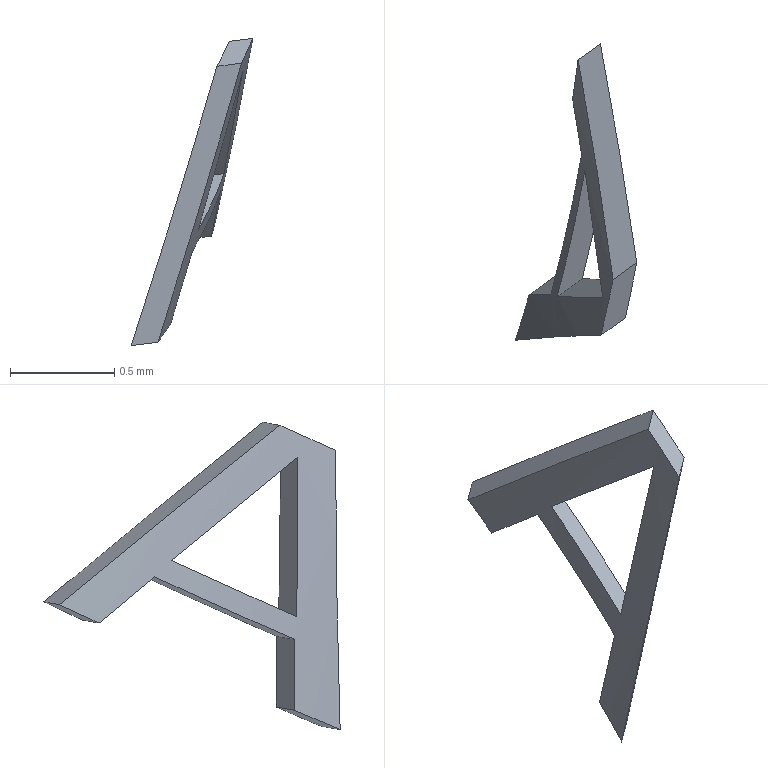Part | SolidWorks | features BaseBody 1 | 1 solid | 13 faces | box 0.5835 x 1.422 x 1.475 mm | volume 0.05932 mm3 | plane 11 | cylinder 2 | commonest cylinder face diameters 16.8 x1 17 x1
STEP:
#1=CARTESIAN_POINT('',(1974.921,-245.366,992.482));
#2=VERTEX_POINT('',#1);
#3=CARTESIAN_POINT('',(1974.98,-245.098,992.601));
#4=VERTEX_POINT('',#3);
#5=CARTESIAN_POINT('',(1966.892,-244.458,994.777));
#6=DIRECTION('',(0.2015,-0.436,0.8771));
#7=DIRECTION('',(-0.7309,-0.6631,-0.1618));
#8=AXIS2_PLACEMENT_3D('',#5,#6,#7);
#9=CIRCLE('',#8,8.4);
#10=EDGE_CURVE('',#2,#4,#9,.T.);
#11=ORIENTED_EDGE('',*,*,#10,.T.);
#12=CARTESIAN_POINT('',(1974.812,-244.041,991.74));
#13=VERTEX_POINT('',#12);
#14=CARTESIAN_POINT('',(1974.98,-245.098,992.601));
#15=CARTESIAN_POINT('',(1974.932,-244.742,992.317));
#16=CARTESIAN_POINT('',(1974.875,-244.39,992.03));
#17=CARTESIAN_POINT('',(1974.812,-244.041,991.74));
#18=B_SPLINE_CURVE_WITH_KNOTS('',3,(#14,#15,#16,#17),.UNSPECIFIED.,.F.,.F.,(4,4),(0.,1.),.UNSPECIFIED.);
#19=EDGE_CURVE('',#4,#13,#18,.T.);
#20=ORIENTED_EDGE('',*,*,#19,.T.);
#21=CARTESIAN_POINT('',(1974.785,-244.229,991.653));
#22=VERTEX_POINT('',#21);
#23=CARTESIAN_POINT('',(1966.64,-243.913,993.681));
#24=DIRECTION('',(-0.2015,0.436,-0.8771));
#25=DIRECTION('',(-0.7309,-0.6631,-0.1618));
#26=AXIS2_PLACEMENT_3D('',#23,#24,#25);
#27=CIRCLE('',#26,8.4);
#28=EDGE_CURVE('',#13,#22,#27,.T.);
#29=ORIENTED_EDGE('',*,*,#28,.T.);
#30=CARTESIAN_POINT('',(1974.829,-244.496,991.874));
#31=VERTEX_POINT('',#30);
#32=CARTESIAN_POINT('',(1974.829,-244.496,991.874));
#33=CARTESIAN_POINT('',(1974.815,-244.407,991.8));
#34=CARTESIAN_POINT('',(1974.8,-244.318,991.726));
#35=CARTESIAN_POINT('',(1974.785,-244.229,991.653));
#36=B_SPLINE_CURVE_WITH_KNOTS('',3,(#32,#33,#34,#35),.UNSPECIFIED.,.F.,.F.,(4,4),(0.,1.),.UNSPECIFIED.);
#37=EDGE_CURVE('',#31,#22,#36,.T.);
#38=ORIENTED_EDGE('',*,*,#37,.F.);
#39=CARTESIAN_POINT('',(1974.681,-245.167,991.574));
#40=VERTEX_POINT('',#39);
#41=CARTESIAN_POINT('',(1966.704,-244.052,993.961));
#42=DIRECTION('',(-0.2015,0.436,-0.8771));
#43=DIRECTION('',(-0.7309,-0.6631,-0.1618));
#44=AXIS2_PLACEMENT_3D('',#41,#42,#43);
#45=CIRCLE('',#44,8.4);
#46=EDGE_CURVE('',#31,#40,#45,.T.);
#47=ORIENTED_EDGE('',*,*,#46,.T.);
#48=CARTESIAN_POINT('',(1974.577,-245.169,991.233));
#49=VERTEX_POINT('',#48);
#50=CARTESIAN_POINT('',(1974.577,-245.169,991.233));
#51=CARTESIAN_POINT('',(1974.612,-245.168,991.347));
#52=CARTESIAN_POINT('',(1974.647,-245.168,991.46));
#53=CARTESIAN_POINT('',(1974.681,-245.167,991.574));
#54=B_SPLINE_CURVE_WITH_KNOTS('',3,(#50,#51,#52,#53),.UNSPECIFIED.,.F.,.F.,(4,4),(0.,1.),.UNSPECIFIED.);
#55=EDGE_CURVE('',#49,#40,#54,.T.);
#56=ORIENTED_EDGE('',*,*,#55,.F.);
#57=CARTESIAN_POINT('',(1974.51,-245.387,991.14));
#58=VERTEX_POINT('',#57);
#59=CARTESIAN_POINT('',(1966.64,-243.913,993.681));
#60=DIRECTION('',(-0.2015,0.436,-0.8771));
#61=DIRECTION('',(-0.7309,-0.6631,-0.1618));
#62=AXIS2_PLACEMENT_3D('',#59,#60,#61);
#63=CIRCLE('',#62,8.4);
#64=EDGE_CURVE('',#49,#58,#63,.T.);
#65=ORIENTED_EDGE('',*,*,#64,.T.);
#66=CARTESIAN_POINT('',(1974.51,-245.387,991.14));
#67=CARTESIAN_POINT('',(1974.656,-245.372,991.584));
#68=CARTESIAN_POINT('',(1974.793,-245.366,992.032));
#69=CARTESIAN_POINT('',(1974.921,-245.366,992.482));
#70=B_SPLINE_CURVE_WITH_KNOTS('',3,(#66,#67,#68,#69),.UNSPECIFIED.,.F.,.F.,(4,4),(0.,1.),.UNSPECIFIED.);
#71=EDGE_CURVE('',#58,#2,#70,.T.);
#72=ORIENTED_EDGE('',*,*,#71,.T.);
#73=EDGE_LOOP('',(#11,#20,#29,#38,#47,#56,#65,#72));
#74=FACE_OUTER_BOUND('',#73,.T.);
#75=CARTESIAN_POINT('',(1974.931,-245.184,992.448));
#76=VERTEX_POINT('',#75);
#77=CARTESIAN_POINT('',(1974.845,-244.575,991.952));
#78=VERTEX_POINT('',#77);
#79=CARTESIAN_POINT('',(1974.931,-245.184,992.448));
#80=CARTESIAN_POINT('',(1974.905,-244.98,992.284));
#81=CARTESIAN_POINT('',(1974.876,-244.777,992.118));
#82=CARTESIAN_POINT('',(1974.845,-244.575,991.952));
#83=B_SPLINE_CURVE_WITH_KNOTS('',3,(#79,#80,#81,#82),.UNSPECIFIED.,.F.,.F.,(4,4),(0.,1.),.UNSPECIFIED.);
#84=EDGE_CURVE('',#76,#78,#83,.T.);
#85=ORIENTED_EDGE('',*,*,#84,.F.);
#86=CARTESIAN_POINT('',(1974.712,-245.179,991.683));
#87=VERTEX_POINT('',#86);
#88=CARTESIAN_POINT('',(1974.712,-245.179,991.683));
#89=CARTESIAN_POINT('',(1974.787,-245.178,991.937));
#90=CARTESIAN_POINT('',(1974.86,-245.18,992.192));
#91=CARTESIAN_POINT('',(1974.931,-245.184,992.448));
#92=B_SPLINE_CURVE_WITH_KNOTS('',3,(#88,#89,#90,#91),.UNSPECIFIED.,.F.,.F.,(4,4),(0.,1.),.UNSPECIFIED.);
#93=EDGE_CURVE('',#87,#76,#92,.T.);
#94=ORIENTED_EDGE('',*,*,#93,.F.);
#95=CARTESIAN_POINT('',(1966.726,-244.099,994.054));
#96=DIRECTION('',(-0.2015,0.436,-0.8771));
#97=DIRECTION('',(-0.7309,-0.6631,-0.1618));
#98=AXIS2_PLACEMENT_3D('',#95,#96,#97);
#99=CIRCLE('',#98,8.4);
#100=EDGE_CURVE('',#78,#87,#99,.T.);
#101=ORIENTED_EDGE('',*,*,#100,.F.);
#102=EDGE_LOOP('',(#85,#94,#101));
#103=FACE_BOUND('',#102,.T.);
#104=CARTESIAN_POINT('',(1967.45,-245.666,997.207));
#105=DIRECTION('',(0.2015,-0.436,0.8771));
#106=DIRECTION('',(-0.7309,-0.6631,-0.1618));
#107=AXIS2_PLACEMENT_3D('',#104,#105,#106);
#108=CYLINDRICAL_SURFACE('',#107,8.4);
#109=ADVANCED_FACE('',(#74,#103),#108,.F.);
#110=CARTESIAN_POINT('',(1975.039,-245.282,992.496));
#111=VERTEX_POINT('',#110);
#112=CARTESIAN_POINT('',(1974.98,-245.324,992.489));
#113=DIRECTION('',(-0.8088,-0.5792,-0.1022));
#114=VECTOR('',#113,1000.);
#115=LINE('',#112,#114);
#116=EDGE_CURVE('',#111,#2,#115,.T.);
#117=ORIENTED_EDGE('',*,*,#116,.T.);
#118=ORIENTED_EDGE('',*,*,#71,.F.);
#119=CARTESIAN_POINT('',(1974.638,-245.295,991.157));
#120=VERTEX_POINT('',#119);
#121=CARTESIAN_POINT('',(1974.574,-245.341,991.149));
#122=DIRECTION('',(-0.8088,-0.5792,-0.1022));
#123=VECTOR('',#122,1000.);
#124=LINE('',#121,#123);
#125=EDGE_CURVE('',#120,#58,#124,.T.);
#126=ORIENTED_EDGE('',*,*,#125,.F.);
#127=CARTESIAN_POINT('',(1974.638,-245.295,991.157));
#128=CARTESIAN_POINT('',(1974.723,-245.288,991.423));
#129=CARTESIAN_POINT('',(1974.806,-245.283,991.69));
#130=CARTESIAN_POINT('',(1974.886,-245.281,991.958));
#131=CARTESIAN_POINT('',(1974.963,-245.28,992.227));
#132=CARTESIAN_POINT('',(1975.039,-245.282,992.496));
#133=B_SPLINE_CURVE_WITH_KNOTS('',5,(#127,#128,#129,#130,#131,#132),.UNSPECIFIED.,.F.,.F.,(6,6),(0.,1.),.UNSPECIFIED.);
#134=EDGE_CURVE('',#120,#111,#133,.T.);
#135=ORIENTED_EDGE('',*,*,#134,.T.);
#136=EDGE_LOOP('',(#117,#118,#126,#135));
#137=FACE_OUTER_BOUND('',#136,.T.);
#138=CARTESIAN_POINT('',(1982.394,-239.741,992.136));
#139=DIRECTION('',(0.5879,-0.7913,-0.1679));
#140=DIRECTION('',(-0.01639,0.1959,-0.9805));
#141=AXIS2_PLACEMENT_3D('',#138,#139,#140);
#142=PLANE('',#141);
#143=ADVANCED_FACE('',(#137),#142,.T.);
#144=ORIENTED_EDGE('',*,*,#125,.T.);
#145=ORIENTED_EDGE('',*,*,#64,.F.);
#146=CARTESIAN_POINT('',(1974.701,-245.081,991.249));
#147=VERTEX_POINT('',#146);
#148=CARTESIAN_POINT('',(1974.639,-245.125,991.241));
#149=DIRECTION('',(-0.8088,-0.5792,-0.1022));
#150=VECTOR('',#149,1000.);
#151=LINE('',#148,#150);
#152=EDGE_CURVE('',#147,#49,#151,.T.);
#153=ORIENTED_EDGE('',*,*,#152,.F.);
#154=CARTESIAN_POINT('',(1966.64,-243.913,993.681));
#155=DIRECTION('',(-0.2015,0.436,-0.8771));
#156=DIRECTION('',(-0.7309,-0.6631,-0.1618));
#157=AXIS2_PLACEMENT_3D('',#154,#155,#156);
#158=CIRCLE('',#157,8.5);
#159=EDGE_CURVE('',#147,#120,#158,.T.);
#160=ORIENTED_EDGE('',*,*,#159,.T.);
#161=EDGE_LOOP('',(#144,#145,#153,#160));
#162=FACE_OUTER_BOUND('',#161,.T.);
#163=CARTESIAN_POINT('',(1982.308,-239.633,992.21));
#164=DIRECTION('',(-0.2015,0.436,-0.8771));
#165=DIRECTION('',(-0.5526,0.6888,0.4693));
#166=AXIS2_PLACEMENT_3D('',#163,#164,#165);
#167=PLANE('',#166);
#168=ADVANCED_FACE('',(#162),#167,.T.);
#169=ORIENTED_EDGE('',*,*,#152,.T.);
#170=ORIENTED_EDGE('',*,*,#55,.T.);
#171=CARTESIAN_POINT('',(1974.802,-245.08,991.589));
#172=VERTEX_POINT('',#171);
#173=CARTESIAN_POINT('',(1974.741,-245.124,991.582));
#174=DIRECTION('',(-0.8088,-0.5792,-0.1022));
#175=VECTOR('',#174,1000.);
#176=LINE('',#173,#175);
#177=EDGE_CURVE('',#172,#40,#176,.T.);
#178=ORIENTED_EDGE('',*,*,#177,.F.);
#179=CARTESIAN_POINT('',(1974.701,-245.081,991.249));
#180=CARTESIAN_POINT('',(1974.721,-245.08,991.317));
#181=CARTESIAN_POINT('',(1974.742,-245.08,991.385));
#182=CARTESIAN_POINT('',(1974.762,-245.08,991.453));
#183=CARTESIAN_POINT('',(1974.782,-245.08,991.521));
#184=CARTESIAN_POINT('',(1974.802,-245.08,991.589));
#185=B_SPLINE_CURVE_WITH_KNOTS('',5,(#179,#180,#181,#182,#183,#184),.UNSPECIFIED.,.F.,.F.,(6,6),(0.,1.),.UNSPECIFIED.);
#186=EDGE_CURVE('',#147,#172,#185,.T.);
#187=ORIENTED_EDGE('',*,*,#186,.F.);
#188=EDGE_LOOP('',(#169,#170,#178,#187));
#189=FACE_OUTER_BOUND('',#188,.T.);
#190=CARTESIAN_POINT('',(1982.314,-239.7,992.539));
#191=DIRECTION('',(-0.5878,0.7901,0.174));
#192=DIRECTION('',(0.02007,-0.2008,0.9794));
#193=AXIS2_PLACEMENT_3D('',#190,#191,#192);
#194=PLANE('',#193);
#195=ADVANCED_FACE('',(#189),#194,.T.);
#196=ORIENTED_EDGE('',*,*,#177,.T.);
#197=ORIENTED_EDGE('',*,*,#46,.F.);
#198=CARTESIAN_POINT('',(1974.94,-244.417,991.888));
#199=VERTEX_POINT('',#198);
#200=CARTESIAN_POINT('',(1974.884,-244.457,991.881));
#201=DIRECTION('',(-0.8088,-0.5792,-0.1022));
#202=VECTOR('',#201,1000.);
#203=LINE('',#200,#202);
#204=EDGE_CURVE('',#199,#31,#203,.T.);
#205=ORIENTED_EDGE('',*,*,#204,.F.);
#206=CARTESIAN_POINT('',(1966.704,-244.052,993.961));
#207=DIRECTION('',(-0.2015,0.436,-0.8771));
#208=DIRECTION('',(-0.7309,-0.6631,-0.1618));
#209=AXIS2_PLACEMENT_3D('',#206,#207,#208);
#210=CIRCLE('',#209,8.5);
#211=EDGE_CURVE('',#199,#172,#210,.T.);
#212=ORIENTED_EDGE('',*,*,#211,.T.);
#213=EDGE_LOOP('',(#196,#197,#205,#212));
#214=FACE_OUTER_BOUND('',#213,.T.);
#215=CARTESIAN_POINT('',(1982.026,-239.342,992.783));
#216=DIRECTION('',(-0.2015,0.436,-0.8771));
#217=DIRECTION('',(-0.5526,0.6888,0.4693));
#218=AXIS2_PLACEMENT_3D('',#215,#216,#217);
#219=PLANE('',#218);
#220=ADVANCED_FACE('',(#214),#219,.T.);
#221=ORIENTED_EDGE('',*,*,#204,.T.);
#222=ORIENTED_EDGE('',*,*,#37,.T.);
#223=CARTESIAN_POINT('',(1974.895,-244.151,991.666));
#224=VERTEX_POINT('',#223);
#225=CARTESIAN_POINT('',(1974.84,-244.19,991.659));
#226=DIRECTION('',(-0.8088,-0.5792,-0.1022));
#227=VECTOR('',#226,1000.);
#228=LINE('',#225,#227);
#229=EDGE_CURVE('',#224,#22,#228,.T.);
#230=ORIENTED_EDGE('',*,*,#229,.F.);
#231=CARTESIAN_POINT('',(1974.94,-244.417,991.888));
#232=CARTESIAN_POINT('',(1974.931,-244.364,991.844));
#233=CARTESIAN_POINT('',(1974.922,-244.31,991.799));
#234=CARTESIAN_POINT('',(1974.913,-244.257,991.755));
#235=CARTESIAN_POINT('',(1974.904,-244.204,991.711));
#236=CARTESIAN_POINT('',(1974.895,-244.151,991.666));
#237=B_SPLINE_CURVE_WITH_KNOTS('',5,(#231,#232,#233,#234,#235,#236),.UNSPECIFIED.,.F.,.F.,(6,6),(0.,1.),.UNSPECIFIED.);
#238=EDGE_CURVE('',#199,#224,#237,.T.);
#239=ORIENTED_EDGE('',*,*,#238,.F.);
#240=EDGE_LOOP('',(#221,#222,#230,#239));
#241=FACE_OUTER_BOUND('',#240,.T.);
#242=CARTESIAN_POINT('',(1981.905,-239.131,992.552));
#243=DIRECTION('',(0.4628,-0.5195,-0.7183));
#244=DIRECTION('',(-0.363,0.6282,-0.6882));
#245=AXIS2_PLACEMENT_3D('',#242,#243,#244);
#246=PLANE('',#245);
#247=ADVANCED_FACE('',(#241),#246,.T.);
#248=ORIENTED_EDGE('',*,*,#229,.T.);
#249=ORIENTED_EDGE('',*,*,#28,.F.);
#250=CARTESIAN_POINT('',(1974.919,-243.964,991.754));
#251=VERTEX_POINT('',#250);
#252=CARTESIAN_POINT('',(1974.865,-244.003,991.747));
#253=DIRECTION('',(-0.8088,-0.5792,-0.1022));
#254=VECTOR('',#253,1000.);
#255=LINE('',#252,#254);
#256=EDGE_CURVE('',#251,#13,#255,.T.);
#257=ORIENTED_EDGE('',*,*,#256,.F.);
#258=CARTESIAN_POINT('',(1966.64,-243.913,993.681));
#259=DIRECTION('',(-0.2015,0.436,-0.8771));
#260=DIRECTION('',(-0.7309,-0.6631,-0.1618));
#261=AXIS2_PLACEMENT_3D('',#258,#259,#260);
#262=CIRCLE('',#261,8.5);
#263=EDGE_CURVE('',#251,#224,#262,.T.);
#264=ORIENTED_EDGE('',*,*,#263,.T.);
#265=EDGE_LOOP('',(#248,#249,#257,#264));
#266=FACE_OUTER_BOUND('',#265,.T.);
#267=CARTESIAN_POINT('',(1982.308,-239.633,992.21));
#268=DIRECTION('',(-0.2015,0.436,-0.8771));
#269=DIRECTION('',(-0.5526,0.6888,0.4693));
#270=AXIS2_PLACEMENT_3D('',#267,#268,#269);
#271=PLANE('',#270);
#272=ADVANCED_FACE('',(#266),#271,.T.);
#273=ORIENTED_EDGE('',*,*,#256,.T.);
#274=ORIENTED_EDGE('',*,*,#19,.F.);
#275=CARTESIAN_POINT('',(1975.094,-245.016,992.616));
#276=VERTEX_POINT('',#275);
#277=CARTESIAN_POINT('',(1975.037,-245.057,992.608));
#278=DIRECTION('',(-0.8088,-0.5792,-0.1022));
#279=VECTOR('',#278,1000.);
#280=LINE('',#277,#279);
#281=EDGE_CURVE('',#276,#4,#280,.T.);
#282=ORIENTED_EDGE('',*,*,#281,.F.);
#283=CARTESIAN_POINT('',(1975.094,-245.016,992.616));
#284=CARTESIAN_POINT('',(1975.063,-244.804,992.445));
#285=CARTESIAN_POINT('',(1975.03,-244.593,992.273));
#286=CARTESIAN_POINT('',(1974.995,-244.382,992.1));
#287=CARTESIAN_POINT('',(1974.958,-244.173,991.927));
#288=CARTESIAN_POINT('',(1974.919,-243.964,991.754));
#289=B_SPLINE_CURVE_WITH_KNOTS('',5,(#283,#284,#285,#286,#287,#288),.UNSPECIFIED.,.F.,.F.,(6,6),(0.,1.),.UNSPECIFIED.);
#290=EDGE_CURVE('',#276,#251,#289,.T.);
#291=ORIENTED_EDGE('',*,*,#290,.T.);
#292=EDGE_LOOP('',(#273,#274,#282,#291));
#293=FACE_OUTER_BOUND('',#292,.T.);
#294=CARTESIAN_POINT('',(1982.3,-239.855,993.526));
#295=DIRECTION('',(-0.4605,0.5155,0.7226));
#296=DIRECTION('',(0.3659,-0.6315,0.6837));
#297=AXIS2_PLACEMENT_3D('',#294,#295,#296);
#298=PLANE('',#297);
#299=ADVANCED_FACE('',(#293),#298,.T.);
#300=ORIENTED_EDGE('',*,*,#281,.T.);
#301=ORIENTED_EDGE('',*,*,#10,.F.);
#302=ORIENTED_EDGE('',*,*,#116,.F.);
#303=CARTESIAN_POINT('',(1966.892,-244.458,994.777));
#304=DIRECTION('',(0.2015,-0.436,0.8771));
#305=DIRECTION('',(-0.7309,-0.6631,-0.1618));
#306=AXIS2_PLACEMENT_3D('',#303,#304,#305);
#307=CIRCLE('',#306,8.5);
#308=EDGE_CURVE('',#111,#276,#307,.T.);
#309=ORIENTED_EDGE('',*,*,#308,.T.);
#310=EDGE_LOOP('',(#300,#301,#302,#309));
#311=FACE_OUTER_BOUND('',#310,.T.);
#312=CARTESIAN_POINT('',(1982.415,-239.999,993.428));
#313=DIRECTION('',(0.2015,-0.436,0.8771));
#314=DIRECTION('',(0.5526,-0.6888,-0.4693));
#315=AXIS2_PLACEMENT_3D('',#312,#313,#314);
#316=PLANE('',#315);
#317=ADVANCED_FACE('',(#311),#316,.T.);
#318=CARTESIAN_POINT('',(1974.956,-244.495,991.966));
#319=VERTEX_POINT('',#318);
#320=CARTESIAN_POINT('',(1974.832,-245.092,991.698));
#321=VERTEX_POINT('',#320);
#322=CARTESIAN_POINT('',(1966.726,-244.099,994.054));
#323=DIRECTION('',(-0.2015,0.436,-0.8771));
#324=DIRECTION('',(-0.7309,-0.6631,-0.1618));
#325=AXIS2_PLACEMENT_3D('',#322,#323,#324);
#326=CIRCLE('',#325,8.5);
#327=EDGE_CURVE('',#319,#321,#326,.T.);
#328=ORIENTED_EDGE('',*,*,#327,.F.);
#329=CARTESIAN_POINT('',(1974.9,-244.535,991.959));
#330=DIRECTION('',(-0.8088,-0.5792,-0.1022));
#331=VECTOR('',#330,1000.);
#332=LINE('',#329,#331);
#333=EDGE_CURVE('',#319,#78,#332,.T.);
#334=ORIENTED_EDGE('',*,*,#333,.T.);
#335=ORIENTED_EDGE('',*,*,#100,.T.);
#336=CARTESIAN_POINT('',(1974.772,-245.135,991.69));
#337=DIRECTION('',(-0.8088,-0.5792,-0.1022));
#338=VECTOR('',#337,1000.);
#339=LINE('',#336,#338);
#340=EDGE_CURVE('',#321,#87,#339,.T.);
#341=ORIENTED_EDGE('',*,*,#340,.F.);
#342=EDGE_LOOP('',(#328,#334,#335,#341));
#343=FACE_OUTER_BOUND('',#342,.T.);
#344=CARTESIAN_POINT('',(1982.062,-239.406,992.864));
#345=DIRECTION('',(-0.2015,0.436,-0.8771));
#346=DIRECTION('',(-0.5526,0.6888,0.4693));
#347=AXIS2_PLACEMENT_3D('',#344,#345,#346);
#348=PLANE('',#347);
#349=ADVANCED_FACE('',(#343),#348,.F.);
#350=CARTESIAN_POINT('',(1975.046,-245.102,992.463));
#351=VERTEX_POINT('',#350);
#352=CARTESIAN_POINT('',(1974.832,-245.092,991.698));
#353=CARTESIAN_POINT('',(1974.876,-245.093,991.851));
#354=CARTESIAN_POINT('',(1974.92,-245.094,992.003));
#355=CARTESIAN_POINT('',(1974.963,-245.096,992.156));
#356=CARTESIAN_POINT('',(1975.005,-245.099,992.31));
#357=CARTESIAN_POINT('',(1975.046,-245.102,992.463));
#358=B_SPLINE_CURVE_WITH_KNOTS('',5,(#352,#353,#354,#355,#356,#357),.UNSPECIFIED.,.F.,.F.,(6,6),(0.,1.),.UNSPECIFIED.);
#359=EDGE_CURVE('',#321,#351,#358,.T.);
#360=ORIENTED_EDGE('',*,*,#359,.F.);
#361=ORIENTED_EDGE('',*,*,#340,.T.);
#362=ORIENTED_EDGE('',*,*,#93,.T.);
#363=CARTESIAN_POINT('',(1974.988,-245.143,992.456));
#364=DIRECTION('',(-0.8088,-0.5792,-0.1022));
#365=VECTOR('',#364,1000.);
#366=LINE('',#363,#365);
#367=EDGE_CURVE('',#351,#76,#366,.T.);
#368=ORIENTED_EDGE('',*,*,#367,.F.);
#369=EDGE_LOOP('',(#360,#361,#362,#368));
#370=FACE_OUTER_BOUND('',#369,.T.);
#371=CARTESIAN_POINT('',(1982.321,-239.729,992.644));
#372=DIRECTION('',(0.5878,-0.7901,-0.174));
#373=DIRECTION('',(-0.02007,0.2008,-0.9794));
#374=AXIS2_PLACEMENT_3D('',#371,#372,#373);
#375=PLANE('',#374);
#376=ADVANCED_FACE('',(#370),#375,.F.);
#377=CARTESIAN_POINT('',(1975.046,-245.102,992.463));
#378=CARTESIAN_POINT('',(1975.03,-244.98,992.364));
#379=CARTESIAN_POINT('',(1975.012,-244.858,992.265));
#380=CARTESIAN_POINT('',(1974.994,-244.737,992.166));
#381=CARTESIAN_POINT('',(1974.975,-244.616,992.066));
#382=CARTESIAN_POINT('',(1974.956,-244.495,991.966));
#383=B_SPLINE_CURVE_WITH_KNOTS('',5,(#377,#378,#379,#380,#381,#382),.UNSPECIFIED.,.F.,.F.,(6,6),(0.,1.),.UNSPECIFIED.);
#384=EDGE_CURVE('',#351,#319,#383,.T.);
#385=ORIENTED_EDGE('',*,*,#384,.F.);
#386=ORIENTED_EDGE('',*,*,#367,.T.);
#387=ORIENTED_EDGE('',*,*,#84,.T.);
#388=ORIENTED_EDGE('',*,*,#333,.F.);
#389=EDGE_LOOP('',(#385,#386,#387,#388));
#390=FACE_OUTER_BOUND('',#389,.T.);
#391=CARTESIAN_POINT('',(1982.336,-239.881,993.384));
#392=DIRECTION('',(-0.4628,0.5195,0.7183));
#393=DIRECTION('',(0.363,-0.6282,0.6882));
#394=AXIS2_PLACEMENT_3D('',#391,#392,#393);
#395=PLANE('',#394);
#396=ADVANCED_FACE('',(#390),#395,.F.);
#397=ORIENTED_EDGE('',*,*,#134,.F.);
#398=ORIENTED_EDGE('',*,*,#159,.F.);
#399=ORIENTED_EDGE('',*,*,#186,.T.);
#400=ORIENTED_EDGE('',*,*,#211,.F.);
#401=ORIENTED_EDGE('',*,*,#238,.T.);
#402=ORIENTED_EDGE('',*,*,#263,.F.);
#403=ORIENTED_EDGE('',*,*,#290,.F.);
#404=ORIENTED_EDGE('',*,*,#308,.F.);
#405=EDGE_LOOP('',(#397,#398,#399,#400,#401,#402,#403,#404));
#406=FACE_OUTER_BOUND('',#405,.T.);
#407=ORIENTED_EDGE('',*,*,#384,.T.);
#408=ORIENTED_EDGE('',*,*,#327,.T.);
#409=ORIENTED_EDGE('',*,*,#359,.T.);
#410=EDGE_LOOP('',(#407,#408,#409));
#411=FACE_BOUND('',#410,.T.);
#412=CARTESIAN_POINT('',(1967.45,-245.666,997.207));
#413=DIRECTION('',(0.2015,-0.436,0.8771));
#414=DIRECTION('',(-0.7309,-0.6631,-0.1618));
#415=AXIS2_PLACEMENT_3D('',#412,#413,#414);
#416=CYLINDRICAL_SURFACE('',#415,8.5);
#417=ADVANCED_FACE('',(#406,#411),#416,.T.);
#418=CLOSED_SHELL('',(#109,#143,#168,#195,#220,#247,#272,#299,#317,#349,#376,#396,#417));
#419=MANIFOLD_SOLID_BREP('',#418);
#420=CARTESIAN_POINT('',(0.,0.,0.));
#421=DIRECTION('',(0.,0.,1.));
#422=DIRECTION('',(1.,0.,0.));
#423=AXIS2_PLACEMENT_3D('',#420,#421,#422);
#424=(LENGTH_UNIT()NAMED_UNIT(*)SI_UNIT(.MILLI.,.METRE.));
#425=UNCERTAINTY_MEASURE_WITH_UNIT(LENGTH_MEASURE(0.00001),#424,'','');
#426=(NAMED_UNIT(*)PLANE_ANGLE_UNIT()SI_UNIT($,.RADIAN.));
#427=(NAMED_UNIT(*)SI_UNIT($,.STERADIAN.)SOLID_ANGLE_UNIT());
#428=(GEOMETRIC_REPRESENTATION_CONTEXT(3)GLOBAL_UNCERTAINTY_ASSIGNED_CONTEXT((#425))GLOBAL_UNIT_ASSIGNED_CONTEXT((#424,#426,#427))REPRESENTATION_CONTEXT('',''));
#429=ADVANCED_BREP_SHAPE_REPRESENTATION('',(#419,#423),#428);